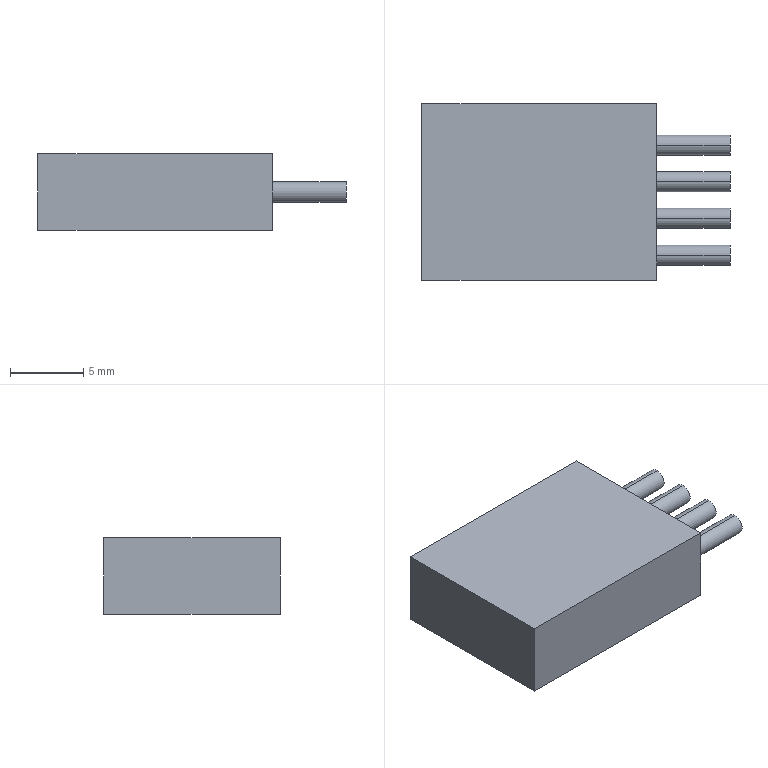Part | NX | features BREP 1 | 1 solid | 18 faces | box 21 x 12 x 5.2 mm | volume 1028 mm3 | plane 10 | cylinder 8 | commonest cylinder face diameters 1.375 x8
STEP:
#1=CARTESIAN_POINT('',(21.,1.7,3.287));
#2=VERTEX_POINT('',#1);
#3=CARTESIAN_POINT('',(21.,1.7,1.913));
#4=VERTEX_POINT('',#3);
#5=CARTESIAN_POINT('',(21.,1.7,2.6));
#6=DIRECTION('',(1.,0.,0.));
#7=DIRECTION('',(0.,0.,-1.));
#8=AXIS2_PLACEMENT_3D('',#5,#6,#7);
#9=CIRCLE('',#8,0.6873);
#10=EDGE_CURVE('',#2,#4,#9,.T.);
#11=ORIENTED_EDGE('',*,*,#10,.T.);
#12=CARTESIAN_POINT('',(21.,1.7,2.6));
#13=DIRECTION('',(1.,0.,0.));
#14=DIRECTION('',(0.,0.,-1.));
#15=AXIS2_PLACEMENT_3D('',#12,#13,#14);
#16=CIRCLE('',#15,0.6873);
#17=EDGE_CURVE('',#4,#2,#16,.T.);
#18=ORIENTED_EDGE('',*,*,#17,.T.);
#19=EDGE_LOOP('',(#11,#18));
#20=FACE_BOUND('',#19,.T.);
#21=CARTESIAN_POINT('',(21.,1.7,2.6));
#22=DIRECTION('',(1.,0.,0.));
#23=DIRECTION('',(0.,0.,-1.));
#24=AXIS2_PLACEMENT_3D('',#21,#22,#23);
#25=PLANE('',#24);
#26=ADVANCED_FACE('',(#20),#25,.T.);
#27=CARTESIAN_POINT('',(16.,1.7,1.913));
#28=VERTEX_POINT('',#27);
#29=CARTESIAN_POINT('',(21.,1.7,1.913));
#30=DIRECTION('',(-1.,0.,0.));
#31=VECTOR('',#30,1000.);
#32=LINE('',#29,#31);
#33=EDGE_CURVE('',#28,#4,#32,.F.);
#34=ORIENTED_EDGE('',*,*,#33,.T.);
#35=ORIENTED_EDGE('',*,*,#10,.F.);
#36=CARTESIAN_POINT('',(16.,1.7,3.287));
#37=VERTEX_POINT('',#36);
#38=CARTESIAN_POINT('',(21.,1.7,3.287));
#39=DIRECTION('',(-1.,0.,0.));
#40=VECTOR('',#39,1000.);
#41=LINE('',#38,#40);
#42=EDGE_CURVE('',#37,#2,#41,.F.);
#43=ORIENTED_EDGE('',*,*,#42,.F.);
#44=CARTESIAN_POINT('',(16.,1.7,2.6));
#45=DIRECTION('',(1.,0.,0.));
#46=DIRECTION('',(0.,0.,1.));
#47=AXIS2_PLACEMENT_3D('',#44,#45,#46);
#48=CIRCLE('',#47,0.6873);
#49=EDGE_CURVE('',#37,#28,#48,.T.);
#50=ORIENTED_EDGE('',*,*,#49,.T.);
#51=EDGE_LOOP('',(#34,#35,#43,#50));
#52=FACE_BOUND('',#51,.T.);
#53=CARTESIAN_POINT('',(21.,1.7,2.6));
#54=DIRECTION('',(-1.,0.,0.));
#55=DIRECTION('',(0.,0.,1.));
#56=AXIS2_PLACEMENT_3D('',#53,#54,#55);
#57=CYLINDRICAL_SURFACE('',#56,0.6873);
#58=ADVANCED_FACE('',(#52),#57,.T.);
#59=CARTESIAN_POINT('',(21.,4.2,3.287));
#60=VERTEX_POINT('',#59);
#61=CARTESIAN_POINT('',(21.,4.2,1.913));
#62=VERTEX_POINT('',#61);
#63=CARTESIAN_POINT('',(21.,4.2,2.6));
#64=DIRECTION('',(1.,0.,0.));
#65=DIRECTION('',(0.,0.,-1.));
#66=AXIS2_PLACEMENT_3D('',#63,#64,#65);
#67=CIRCLE('',#66,0.6873);
#68=EDGE_CURVE('',#60,#62,#67,.T.);
#69=ORIENTED_EDGE('',*,*,#68,.T.);
#70=CARTESIAN_POINT('',(21.,4.2,2.6));
#71=DIRECTION('',(1.,0.,0.));
#72=DIRECTION('',(0.,0.,-1.));
#73=AXIS2_PLACEMENT_3D('',#70,#71,#72);
#74=CIRCLE('',#73,0.6873);
#75=EDGE_CURVE('',#62,#60,#74,.T.);
#76=ORIENTED_EDGE('',*,*,#75,.T.);
#77=EDGE_LOOP('',(#69,#76));
#78=FACE_BOUND('',#77,.T.);
#79=CARTESIAN_POINT('',(21.,4.2,2.6));
#80=DIRECTION('',(1.,0.,0.));
#81=DIRECTION('',(0.,0.,-1.));
#82=AXIS2_PLACEMENT_3D('',#79,#80,#81);
#83=PLANE('',#82);
#84=ADVANCED_FACE('',(#78),#83,.T.);
#85=CARTESIAN_POINT('',(16.,4.2,1.913));
#86=VERTEX_POINT('',#85);
#87=CARTESIAN_POINT('',(21.,4.2,1.913));
#88=DIRECTION('',(-1.,0.,0.));
#89=VECTOR('',#88,1000.);
#90=LINE('',#87,#89);
#91=EDGE_CURVE('',#86,#62,#90,.F.);
#92=ORIENTED_EDGE('',*,*,#91,.T.);
#93=ORIENTED_EDGE('',*,*,#68,.F.);
#94=CARTESIAN_POINT('',(16.,4.2,3.287));
#95=VERTEX_POINT('',#94);
#96=CARTESIAN_POINT('',(21.,4.2,3.287));
#97=DIRECTION('',(-1.,0.,0.));
#98=VECTOR('',#97,1000.);
#99=LINE('',#96,#98);
#100=EDGE_CURVE('',#95,#60,#99,.F.);
#101=ORIENTED_EDGE('',*,*,#100,.F.);
#102=CARTESIAN_POINT('',(16.,4.2,2.6));
#103=DIRECTION('',(1.,0.,0.));
#104=DIRECTION('',(0.,0.,1.));
#105=AXIS2_PLACEMENT_3D('',#102,#103,#104);
#106=CIRCLE('',#105,0.6873);
#107=EDGE_CURVE('',#95,#86,#106,.T.);
#108=ORIENTED_EDGE('',*,*,#107,.T.);
#109=EDGE_LOOP('',(#92,#93,#101,#108));
#110=FACE_BOUND('',#109,.T.);
#111=CARTESIAN_POINT('',(21.,4.2,2.6));
#112=DIRECTION('',(-1.,0.,0.));
#113=DIRECTION('',(0.,0.,1.));
#114=AXIS2_PLACEMENT_3D('',#111,#112,#113);
#115=CYLINDRICAL_SURFACE('',#114,0.6873);
#116=ADVANCED_FACE('',(#110),#115,.T.);
#117=CARTESIAN_POINT('',(21.,6.7,3.287));
#118=VERTEX_POINT('',#117);
#119=CARTESIAN_POINT('',(21.,6.7,1.913));
#120=VERTEX_POINT('',#119);
#121=CARTESIAN_POINT('',(21.,6.7,2.6));
#122=DIRECTION('',(1.,0.,0.));
#123=DIRECTION('',(0.,0.,-1.));
#124=AXIS2_PLACEMENT_3D('',#121,#122,#123);
#125=CIRCLE('',#124,0.6873);
#126=EDGE_CURVE('',#118,#120,#125,.T.);
#127=ORIENTED_EDGE('',*,*,#126,.T.);
#128=CARTESIAN_POINT('',(21.,6.7,2.6));
#129=DIRECTION('',(1.,0.,0.));
#130=DIRECTION('',(0.,0.,-1.));
#131=AXIS2_PLACEMENT_3D('',#128,#129,#130);
#132=CIRCLE('',#131,0.6873);
#133=EDGE_CURVE('',#120,#118,#132,.T.);
#134=ORIENTED_EDGE('',*,*,#133,.T.);
#135=EDGE_LOOP('',(#127,#134));
#136=FACE_BOUND('',#135,.T.);
#137=CARTESIAN_POINT('',(21.,6.7,2.6));
#138=DIRECTION('',(1.,0.,0.));
#139=DIRECTION('',(0.,0.,-1.));
#140=AXIS2_PLACEMENT_3D('',#137,#138,#139);
#141=PLANE('',#140);
#142=ADVANCED_FACE('',(#136),#141,.T.);
#143=CARTESIAN_POINT('',(16.,6.7,1.913));
#144=VERTEX_POINT('',#143);
#145=CARTESIAN_POINT('',(21.,6.7,1.913));
#146=DIRECTION('',(-1.,0.,0.));
#147=VECTOR('',#146,1000.);
#148=LINE('',#145,#147);
#149=EDGE_CURVE('',#144,#120,#148,.F.);
#150=ORIENTED_EDGE('',*,*,#149,.T.);
#151=ORIENTED_EDGE('',*,*,#126,.F.);
#152=CARTESIAN_POINT('',(16.,6.7,3.287));
#153=VERTEX_POINT('',#152);
#154=CARTESIAN_POINT('',(21.,6.7,3.287));
#155=DIRECTION('',(-1.,0.,0.));
#156=VECTOR('',#155,1000.);
#157=LINE('',#154,#156);
#158=EDGE_CURVE('',#153,#118,#157,.F.);
#159=ORIENTED_EDGE('',*,*,#158,.F.);
#160=CARTESIAN_POINT('',(16.,6.7,2.6));
#161=DIRECTION('',(1.,0.,0.));
#162=DIRECTION('',(0.,0.,1.));
#163=AXIS2_PLACEMENT_3D('',#160,#161,#162);
#164=CIRCLE('',#163,0.6873);
#165=EDGE_CURVE('',#153,#144,#164,.T.);
#166=ORIENTED_EDGE('',*,*,#165,.T.);
#167=EDGE_LOOP('',(#150,#151,#159,#166));
#168=FACE_BOUND('',#167,.T.);
#169=CARTESIAN_POINT('',(21.,6.7,2.6));
#170=DIRECTION('',(-1.,0.,0.));
#171=DIRECTION('',(0.,0.,1.));
#172=AXIS2_PLACEMENT_3D('',#169,#170,#171);
#173=CYLINDRICAL_SURFACE('',#172,0.6873);
#174=ADVANCED_FACE('',(#168),#173,.T.);
#175=CARTESIAN_POINT('',(21.,9.2,3.287));
#176=VERTEX_POINT('',#175);
#177=CARTESIAN_POINT('',(21.,9.2,1.913));
#178=VERTEX_POINT('',#177);
#179=CARTESIAN_POINT('',(21.,9.2,2.6));
#180=DIRECTION('',(1.,0.,0.));
#181=DIRECTION('',(0.,0.,-1.));
#182=AXIS2_PLACEMENT_3D('',#179,#180,#181);
#183=CIRCLE('',#182,0.6873);
#184=EDGE_CURVE('',#176,#178,#183,.T.);
#185=ORIENTED_EDGE('',*,*,#184,.T.);
#186=CARTESIAN_POINT('',(21.,9.2,2.6));
#187=DIRECTION('',(1.,0.,0.));
#188=DIRECTION('',(0.,0.,-1.));
#189=AXIS2_PLACEMENT_3D('',#186,#187,#188);
#190=CIRCLE('',#189,0.6873);
#191=EDGE_CURVE('',#178,#176,#190,.T.);
#192=ORIENTED_EDGE('',*,*,#191,.T.);
#193=EDGE_LOOP('',(#185,#192));
#194=FACE_BOUND('',#193,.T.);
#195=CARTESIAN_POINT('',(21.,9.2,2.6));
#196=DIRECTION('',(1.,0.,0.));
#197=DIRECTION('',(0.,0.,-1.));
#198=AXIS2_PLACEMENT_3D('',#195,#196,#197);
#199=PLANE('',#198);
#200=ADVANCED_FACE('',(#194),#199,.T.);
#201=CARTESIAN_POINT('',(16.,9.2,1.913));
#202=VERTEX_POINT('',#201);
#203=CARTESIAN_POINT('',(21.,9.2,1.913));
#204=DIRECTION('',(-1.,0.,0.));
#205=VECTOR('',#204,1000.);
#206=LINE('',#203,#205);
#207=EDGE_CURVE('',#202,#178,#206,.F.);
#208=ORIENTED_EDGE('',*,*,#207,.T.);
#209=ORIENTED_EDGE('',*,*,#184,.F.);
#210=CARTESIAN_POINT('',(16.,9.2,3.287));
#211=VERTEX_POINT('',#210);
#212=CARTESIAN_POINT('',(21.,9.2,3.287));
#213=DIRECTION('',(-1.,0.,0.));
#214=VECTOR('',#213,1000.);
#215=LINE('',#212,#214);
#216=EDGE_CURVE('',#211,#176,#215,.F.);
#217=ORIENTED_EDGE('',*,*,#216,.F.);
#218=CARTESIAN_POINT('',(16.,9.2,2.6));
#219=DIRECTION('',(1.,0.,0.));
#220=DIRECTION('',(0.,0.,1.));
#221=AXIS2_PLACEMENT_3D('',#218,#219,#220);
#222=CIRCLE('',#221,0.6873);
#223=EDGE_CURVE('',#211,#202,#222,.T.);
#224=ORIENTED_EDGE('',*,*,#223,.T.);
#225=EDGE_LOOP('',(#208,#209,#217,#224));
#226=FACE_BOUND('',#225,.T.);
#227=CARTESIAN_POINT('',(21.,9.2,2.6));
#228=DIRECTION('',(-1.,0.,0.));
#229=DIRECTION('',(0.,0.,1.));
#230=AXIS2_PLACEMENT_3D('',#227,#228,#229);
#231=CYLINDRICAL_SURFACE('',#230,0.6873);
#232=ADVANCED_FACE('',(#226),#231,.T.);
#233=CARTESIAN_POINT('',(0.,12.,0.));
#234=VERTEX_POINT('',#233);
#235=CARTESIAN_POINT('',(0.,0.,0.));
#236=VERTEX_POINT('',#235);
#237=CARTESIAN_POINT('',(0.,0.,0.));
#238=DIRECTION('',(0.,-1.,0.));
#239=VECTOR('',#238,1000.);
#240=LINE('',#237,#239);
#241=EDGE_CURVE('',#234,#236,#240,.T.);
#242=ORIENTED_EDGE('',*,*,#241,.F.);
#243=CARTESIAN_POINT('',(16.,12.,0.));
#244=VERTEX_POINT('',#243);
#245=CARTESIAN_POINT('',(0.,12.,0.));
#246=DIRECTION('',(-1.,0.,0.));
#247=VECTOR('',#246,1000.);
#248=LINE('',#245,#247);
#249=EDGE_CURVE('',#244,#234,#248,.T.);
#250=ORIENTED_EDGE('',*,*,#249,.F.);
#251=CARTESIAN_POINT('',(16.,0.,0.));
#252=VERTEX_POINT('',#251);
#253=CARTESIAN_POINT('',(16.,0.,0.));
#254=DIRECTION('',(0.,1.,0.));
#255=VECTOR('',#254,1000.);
#256=LINE('',#253,#255);
#257=EDGE_CURVE('',#252,#244,#256,.T.);
#258=ORIENTED_EDGE('',*,*,#257,.F.);
#259=CARTESIAN_POINT('',(0.,0.,0.));
#260=DIRECTION('',(1.,0.,0.));
#261=VECTOR('',#260,1000.);
#262=LINE('',#259,#261);
#263=EDGE_CURVE('',#236,#252,#262,.T.);
#264=ORIENTED_EDGE('',*,*,#263,.F.);
#265=EDGE_LOOP('',(#242,#250,#258,#264));
#266=FACE_BOUND('',#265,.T.);
#267=CARTESIAN_POINT('',(0.,12.,0.));
#268=DIRECTION('',(0.,0.,-1.));
#269=DIRECTION('',(-1.,0.,0.));
#270=AXIS2_PLACEMENT_3D('',#267,#268,#269);
#271=PLANE('',#270);
#272=ADVANCED_FACE('',(#266),#271,.T.);
#273=CARTESIAN_POINT('',(0.,12.,5.2));
#274=VERTEX_POINT('',#273);
#275=CARTESIAN_POINT('',(0.,0.,5.2));
#276=VERTEX_POINT('',#275);
#277=CARTESIAN_POINT('',(0.,0.,5.2));
#278=DIRECTION('',(0.,-1.,0.));
#279=VECTOR('',#278,1000.);
#280=LINE('',#277,#279);
#281=EDGE_CURVE('',#274,#276,#280,.T.);
#282=ORIENTED_EDGE('',*,*,#281,.T.);
#283=CARTESIAN_POINT('',(16.,0.,5.2));
#284=VERTEX_POINT('',#283);
#285=CARTESIAN_POINT('',(0.,0.,5.2));
#286=DIRECTION('',(1.,0.,0.));
#287=VECTOR('',#286,1000.);
#288=LINE('',#285,#287);
#289=EDGE_CURVE('',#276,#284,#288,.T.);
#290=ORIENTED_EDGE('',*,*,#289,.T.);
#291=CARTESIAN_POINT('',(16.,12.,5.2));
#292=VERTEX_POINT('',#291);
#293=CARTESIAN_POINT('',(16.,0.,5.2));
#294=DIRECTION('',(0.,1.,0.));
#295=VECTOR('',#294,1000.);
#296=LINE('',#293,#295);
#297=EDGE_CURVE('',#284,#292,#296,.T.);
#298=ORIENTED_EDGE('',*,*,#297,.T.);
#299=CARTESIAN_POINT('',(0.,12.,5.2));
#300=DIRECTION('',(-1.,0.,0.));
#301=VECTOR('',#300,1000.);
#302=LINE('',#299,#301);
#303=EDGE_CURVE('',#292,#274,#302,.T.);
#304=ORIENTED_EDGE('',*,*,#303,.T.);
#305=EDGE_LOOP('',(#282,#290,#298,#304));
#306=FACE_BOUND('',#305,.T.);
#307=CARTESIAN_POINT('',(0.,12.,5.2));
#308=DIRECTION('',(0.,0.,-1.));
#309=DIRECTION('',(-1.,0.,0.));
#310=AXIS2_PLACEMENT_3D('',#307,#308,#309);
#311=PLANE('',#310);
#312=ADVANCED_FACE('',(#306),#311,.F.);
#313=ORIENTED_EDGE('',*,*,#249,.T.);
#314=CARTESIAN_POINT('',(0.,12.,5.2));
#315=DIRECTION('',(0.,0.,-1.));
#316=VECTOR('',#315,1000.);
#317=LINE('',#314,#316);
#318=EDGE_CURVE('',#274,#234,#317,.T.);
#319=ORIENTED_EDGE('',*,*,#318,.F.);
#320=ORIENTED_EDGE('',*,*,#303,.F.);
#321=CARTESIAN_POINT('',(16.,12.,5.2));
#322=DIRECTION('',(0.,0.,-1.));
#323=VECTOR('',#322,1000.);
#324=LINE('',#321,#323);
#325=EDGE_CURVE('',#292,#244,#324,.T.);
#326=ORIENTED_EDGE('',*,*,#325,.T.);
#327=EDGE_LOOP('',(#313,#319,#320,#326));
#328=FACE_BOUND('',#327,.T.);
#329=CARTESIAN_POINT('',(0.,12.,5.2));
#330=DIRECTION('',(0.,-1.,0.));
#331=DIRECTION('',(0.,0.,-1.));
#332=AXIS2_PLACEMENT_3D('',#329,#330,#331);
#333=PLANE('',#332);
#334=ADVANCED_FACE('',(#328),#333,.F.);
#335=ORIENTED_EDGE('',*,*,#263,.T.);
#336=CARTESIAN_POINT('',(16.,0.,5.2));
#337=DIRECTION('',(0.,0.,-1.));
#338=VECTOR('',#337,1000.);
#339=LINE('',#336,#338);
#340=EDGE_CURVE('',#284,#252,#339,.T.);
#341=ORIENTED_EDGE('',*,*,#340,.F.);
#342=ORIENTED_EDGE('',*,*,#289,.F.);
#343=CARTESIAN_POINT('',(0.,0.,5.2));
#344=DIRECTION('',(0.,0.,-1.));
#345=VECTOR('',#344,1000.);
#346=LINE('',#343,#345);
#347=EDGE_CURVE('',#276,#236,#346,.T.);
#348=ORIENTED_EDGE('',*,*,#347,.T.);
#349=EDGE_LOOP('',(#335,#341,#342,#348));
#350=FACE_BOUND('',#349,.T.);
#351=CARTESIAN_POINT('',(0.,0.,5.2));
#352=DIRECTION('',(0.,1.,0.));
#353=DIRECTION('',(0.,0.,1.));
#354=AXIS2_PLACEMENT_3D('',#351,#352,#353);
#355=PLANE('',#354);
#356=ADVANCED_FACE('',(#350),#355,.F.);
#357=ORIENTED_EDGE('',*,*,#241,.T.);
#358=ORIENTED_EDGE('',*,*,#347,.F.);
#359=ORIENTED_EDGE('',*,*,#281,.F.);
#360=ORIENTED_EDGE('',*,*,#318,.T.);
#361=EDGE_LOOP('',(#357,#358,#359,#360));
#362=FACE_BOUND('',#361,.T.);
#363=CARTESIAN_POINT('',(0.,0.,5.2));
#364=DIRECTION('',(1.,0.,0.));
#365=DIRECTION('',(0.,0.,-1.));
#366=AXIS2_PLACEMENT_3D('',#363,#364,#365);
#367=PLANE('',#366);
#368=ADVANCED_FACE('',(#362),#367,.F.);
#369=ORIENTED_EDGE('',*,*,#49,.F.);
#370=CARTESIAN_POINT('',(16.,1.7,2.6));
#371=DIRECTION('',(1.,0.,0.));
#372=DIRECTION('',(0.,0.,1.));
#373=AXIS2_PLACEMENT_3D('',#370,#371,#372);
#374=CIRCLE('',#373,0.6873);
#375=EDGE_CURVE('',#28,#37,#374,.T.);
#376=ORIENTED_EDGE('',*,*,#375,.F.);
#377=EDGE_LOOP('',(#369,#376));
#378=FACE_BOUND('',#377,.T.);
#379=ORIENTED_EDGE('',*,*,#165,.F.);
#380=CARTESIAN_POINT('',(16.,6.7,2.6));
#381=DIRECTION('',(1.,0.,0.));
#382=DIRECTION('',(0.,0.,1.));
#383=AXIS2_PLACEMENT_3D('',#380,#381,#382);
#384=CIRCLE('',#383,0.6873);
#385=EDGE_CURVE('',#144,#153,#384,.T.);
#386=ORIENTED_EDGE('',*,*,#385,.F.);
#387=EDGE_LOOP('',(#379,#386));
#388=FACE_BOUND('',#387,.T.);
#389=ORIENTED_EDGE('',*,*,#257,.T.);
#390=ORIENTED_EDGE('',*,*,#325,.F.);
#391=ORIENTED_EDGE('',*,*,#297,.F.);
#392=ORIENTED_EDGE('',*,*,#340,.T.);
#393=EDGE_LOOP('',(#389,#390,#391,#392));
#394=FACE_BOUND('',#393,.T.);
#395=ORIENTED_EDGE('',*,*,#223,.F.);
#396=CARTESIAN_POINT('',(16.,9.2,2.6));
#397=DIRECTION('',(1.,0.,0.));
#398=DIRECTION('',(0.,0.,1.));
#399=AXIS2_PLACEMENT_3D('',#396,#397,#398);
#400=CIRCLE('',#399,0.6873);
#401=EDGE_CURVE('',#202,#211,#400,.T.);
#402=ORIENTED_EDGE('',*,*,#401,.F.);
#403=EDGE_LOOP('',(#395,#402));
#404=FACE_BOUND('',#403,.T.);
#405=ORIENTED_EDGE('',*,*,#107,.F.);
#406=CARTESIAN_POINT('',(16.,4.2,2.6));
#407=DIRECTION('',(1.,0.,0.));
#408=DIRECTION('',(0.,0.,1.));
#409=AXIS2_PLACEMENT_3D('',#406,#407,#408);
#410=CIRCLE('',#409,0.6873);
#411=EDGE_CURVE('',#86,#95,#410,.T.);
#412=ORIENTED_EDGE('',*,*,#411,.F.);
#413=EDGE_LOOP('',(#405,#412));
#414=FACE_BOUND('',#413,.T.);
#415=CARTESIAN_POINT('',(16.,0.,5.2));
#416=DIRECTION('',(-1.,0.,0.));
#417=DIRECTION('',(0.,0.,1.));
#418=AXIS2_PLACEMENT_3D('',#415,#416,#417);
#419=PLANE('',#418);
#420=ADVANCED_FACE('',(#378,#388,#394,#404,#414),#419,.F.);
#421=ORIENTED_EDGE('',*,*,#191,.F.);
#422=ORIENTED_EDGE('',*,*,#207,.F.);
#423=ORIENTED_EDGE('',*,*,#401,.T.);
#424=ORIENTED_EDGE('',*,*,#216,.T.);
#425=EDGE_LOOP('',(#421,#422,#423,#424));
#426=FACE_BOUND('',#425,.T.);
#427=CARTESIAN_POINT('',(21.,9.2,2.6));
#428=DIRECTION('',(-1.,0.,0.));
#429=DIRECTION('',(0.,0.,1.));
#430=AXIS2_PLACEMENT_3D('',#427,#428,#429);
#431=CYLINDRICAL_SURFACE('',#430,0.6873);
#432=ADVANCED_FACE('',(#426),#431,.T.);
#433=ORIENTED_EDGE('',*,*,#133,.F.);
#434=ORIENTED_EDGE('',*,*,#149,.F.);
#435=ORIENTED_EDGE('',*,*,#385,.T.);
#436=ORIENTED_EDGE('',*,*,#158,.T.);
#437=EDGE_LOOP('',(#433,#434,#435,#436));
#438=FACE_BOUND('',#437,.T.);
#439=CARTESIAN_POINT('',(21.,6.7,2.6));
#440=DIRECTION('',(-1.,0.,0.));
#441=DIRECTION('',(0.,0.,1.));
#442=AXIS2_PLACEMENT_3D('',#439,#440,#441);
#443=CYLINDRICAL_SURFACE('',#442,0.6873);
#444=ADVANCED_FACE('',(#438),#443,.T.);
#445=ORIENTED_EDGE('',*,*,#75,.F.);
#446=ORIENTED_EDGE('',*,*,#91,.F.);
#447=ORIENTED_EDGE('',*,*,#411,.T.);
#448=ORIENTED_EDGE('',*,*,#100,.T.);
#449=EDGE_LOOP('',(#445,#446,#447,#448));
#450=FACE_BOUND('',#449,.T.);
#451=CARTESIAN_POINT('',(21.,4.2,2.6));
#452=DIRECTION('',(-1.,0.,0.));
#453=DIRECTION('',(0.,0.,1.));
#454=AXIS2_PLACEMENT_3D('',#451,#452,#453);
#455=CYLINDRICAL_SURFACE('',#454,0.6873);
#456=ADVANCED_FACE('',(#450),#455,.T.);
#457=ORIENTED_EDGE('',*,*,#17,.F.);
#458=ORIENTED_EDGE('',*,*,#33,.F.);
#459=ORIENTED_EDGE('',*,*,#375,.T.);
#460=ORIENTED_EDGE('',*,*,#42,.T.);
#461=EDGE_LOOP('',(#457,#458,#459,#460));
#462=FACE_BOUND('',#461,.T.);
#463=CARTESIAN_POINT('',(21.,1.7,2.6));
#464=DIRECTION('',(-1.,0.,0.));
#465=DIRECTION('',(0.,0.,1.));
#466=AXIS2_PLACEMENT_3D('',#463,#464,#465);
#467=CYLINDRICAL_SURFACE('',#466,0.6873);
#468=ADVANCED_FACE('',(#462),#467,.T.);
#469=CLOSED_SHELL('',(#26,#58,#84,#116,#142,#174,#200,#232,#272,#312,#334,#356,#368,#420,#432,#444,#456,#468));
#470=MANIFOLD_SOLID_BREP('',#469);
#471=(LENGTH_UNIT()NAMED_UNIT(*)SI_UNIT(.MILLI.,.METRE.));
#472=UNCERTAINTY_MEASURE_WITH_UNIT(LENGTH_MEASURE(0.00001),#471,'','');
#473=(NAMED_UNIT(*)PLANE_ANGLE_UNIT()SI_UNIT($,.RADIAN.));
#474=(NAMED_UNIT(*)SI_UNIT($,.STERADIAN.)SOLID_ANGLE_UNIT());
#475=(GEOMETRIC_REPRESENTATION_CONTEXT(3)GLOBAL_UNCERTAINTY_ASSIGNED_CONTEXT((#472))GLOBAL_UNIT_ASSIGNED_CONTEXT((#471,#473,#474))REPRESENTATION_CONTEXT('',''));
#476=ADVANCED_BREP_SHAPE_REPRESENTATION('',(#470),#475);